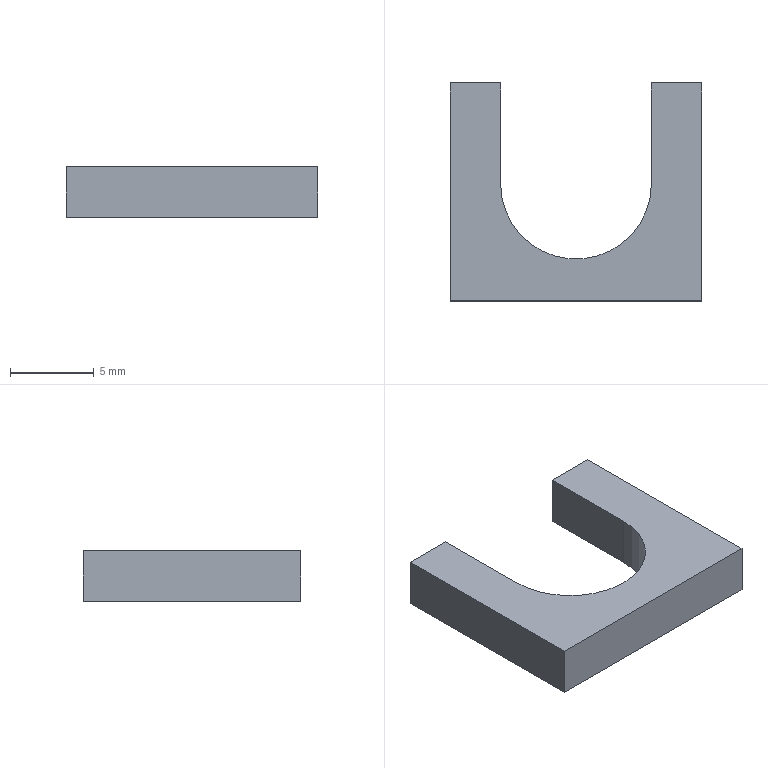Part | NX | features BREP 1 | 1 solid | 10 faces | box 15 x 13 x 3 mm | volume 327.574 mm3 | plane 9 | cylinder 1 | commonest cylinder face diameters 9 x1
STEP:
#1=CARTESIAN_POINT('',(-7.5,13.,0.));
#2=VERTEX_POINT('',#1);
#3=CARTESIAN_POINT('',(-7.5,0.,0.));
#4=VERTEX_POINT('',#3);
#5=CARTESIAN_POINT('',(-7.5,13.,0.));
#6=DIRECTION('',(0.,-1.,0.));
#7=VECTOR('',#6,1000.);
#8=LINE('',#5,#7);
#9=EDGE_CURVE('',#2,#4,#8,.T.);
#10=ORIENTED_EDGE('',*,*,#9,.T.);
#11=CARTESIAN_POINT('',(-7.5,0.,3.));
#12=VERTEX_POINT('',#11);
#13=CARTESIAN_POINT('',(-7.5,0.,3.));
#14=DIRECTION('',(0.,0.,-1.));
#15=VECTOR('',#14,1000.);
#16=LINE('',#13,#15);
#17=EDGE_CURVE('',#12,#4,#16,.T.);
#18=ORIENTED_EDGE('',*,*,#17,.F.);
#19=CARTESIAN_POINT('',(-7.5,13.,3.));
#20=VERTEX_POINT('',#19);
#21=CARTESIAN_POINT('',(-7.5,13.,3.));
#22=DIRECTION('',(0.,-1.,0.));
#23=VECTOR('',#22,1000.);
#24=LINE('',#21,#23);
#25=EDGE_CURVE('',#20,#12,#24,.T.);
#26=ORIENTED_EDGE('',*,*,#25,.F.);
#27=CARTESIAN_POINT('',(-7.5,13.,3.));
#28=DIRECTION('',(0.,0.,-1.));
#29=VECTOR('',#28,1000.);
#30=LINE('',#27,#29);
#31=EDGE_CURVE('',#20,#2,#30,.T.);
#32=ORIENTED_EDGE('',*,*,#31,.T.);
#33=EDGE_LOOP('',(#10,#18,#26,#32));
#34=FACE_BOUND('',#33,.T.);
#35=CARTESIAN_POINT('',(-7.5,13.,3.));
#36=DIRECTION('',(1.,0.,0.));
#37=DIRECTION('',(0.,-1.,0.));
#38=AXIS2_PLACEMENT_3D('',#35,#36,#37);
#39=PLANE('',#38);
#40=ADVANCED_FACE('',(#34),#39,.F.);
#41=CARTESIAN_POINT('',(7.5,0.,0.));
#42=VERTEX_POINT('',#41);
#43=CARTESIAN_POINT('',(-7.5,0.,0.));
#44=DIRECTION('',(1.,0.,0.));
#45=VECTOR('',#44,1000.);
#46=LINE('',#43,#45);
#47=EDGE_CURVE('',#4,#42,#46,.T.);
#48=ORIENTED_EDGE('',*,*,#47,.T.);
#49=CARTESIAN_POINT('',(7.5,0.,3.));
#50=VERTEX_POINT('',#49);
#51=CARTESIAN_POINT('',(7.5,0.,3.));
#52=DIRECTION('',(0.,0.,-1.));
#53=VECTOR('',#52,1000.);
#54=LINE('',#51,#53);
#55=EDGE_CURVE('',#50,#42,#54,.T.);
#56=ORIENTED_EDGE('',*,*,#55,.F.);
#57=CARTESIAN_POINT('',(-7.5,0.,3.));
#58=DIRECTION('',(1.,0.,0.));
#59=VECTOR('',#58,1000.);
#60=LINE('',#57,#59);
#61=EDGE_CURVE('',#12,#50,#60,.T.);
#62=ORIENTED_EDGE('',*,*,#61,.F.);
#63=ORIENTED_EDGE('',*,*,#17,.T.);
#64=EDGE_LOOP('',(#48,#56,#62,#63));
#65=FACE_BOUND('',#64,.T.);
#66=CARTESIAN_POINT('',(-7.5,0.,3.));
#67=DIRECTION('',(0.,1.,0.));
#68=DIRECTION('',(0.,0.,-1.));
#69=AXIS2_PLACEMENT_3D('',#66,#67,#68);
#70=PLANE('',#69);
#71=ADVANCED_FACE('',(#65),#70,.F.);
#72=CARTESIAN_POINT('',(7.5,13.,0.));
#73=VERTEX_POINT('',#72);
#74=CARTESIAN_POINT('',(7.5,0.,0.));
#75=DIRECTION('',(0.,1.,0.));
#76=VECTOR('',#75,1000.);
#77=LINE('',#74,#76);
#78=EDGE_CURVE('',#42,#73,#77,.T.);
#79=ORIENTED_EDGE('',*,*,#78,.T.);
#80=CARTESIAN_POINT('',(7.5,13.,3.));
#81=VERTEX_POINT('',#80);
#82=CARTESIAN_POINT('',(7.5,13.,3.));
#83=DIRECTION('',(0.,0.,-1.));
#84=VECTOR('',#83,1000.);
#85=LINE('',#82,#84);
#86=EDGE_CURVE('',#81,#73,#85,.T.);
#87=ORIENTED_EDGE('',*,*,#86,.F.);
#88=CARTESIAN_POINT('',(7.5,0.,3.));
#89=DIRECTION('',(0.,1.,0.));
#90=VECTOR('',#89,1000.);
#91=LINE('',#88,#90);
#92=EDGE_CURVE('',#50,#81,#91,.T.);
#93=ORIENTED_EDGE('',*,*,#92,.F.);
#94=ORIENTED_EDGE('',*,*,#55,.T.);
#95=EDGE_LOOP('',(#79,#87,#93,#94));
#96=FACE_BOUND('',#95,.T.);
#97=CARTESIAN_POINT('',(7.5,0.,3.));
#98=DIRECTION('',(-1.,0.,0.));
#99=DIRECTION('',(0.,1.,0.));
#100=AXIS2_PLACEMENT_3D('',#97,#98,#99);
#101=PLANE('',#100);
#102=ADVANCED_FACE('',(#96),#101,.F.);
#103=CARTESIAN_POINT('',(4.5,13.,0.));
#104=VERTEX_POINT('',#103);
#105=CARTESIAN_POINT('',(7.5,13.,0.));
#106=DIRECTION('',(-1.,0.,0.));
#107=VECTOR('',#106,1000.);
#108=LINE('',#105,#107);
#109=EDGE_CURVE('',#73,#104,#108,.T.);
#110=ORIENTED_EDGE('',*,*,#109,.T.);
#111=CARTESIAN_POINT('',(4.5,13.,3.));
#112=VERTEX_POINT('',#111);
#113=CARTESIAN_POINT('',(4.5,13.,3.));
#114=DIRECTION('',(0.,0.,-1.));
#115=VECTOR('',#114,1000.);
#116=LINE('',#113,#115);
#117=EDGE_CURVE('',#112,#104,#116,.T.);
#118=ORIENTED_EDGE('',*,*,#117,.F.);
#119=CARTESIAN_POINT('',(7.5,13.,3.));
#120=DIRECTION('',(-1.,0.,0.));
#121=VECTOR('',#120,1000.);
#122=LINE('',#119,#121);
#123=EDGE_CURVE('',#81,#112,#122,.T.);
#124=ORIENTED_EDGE('',*,*,#123,.F.);
#125=ORIENTED_EDGE('',*,*,#86,.T.);
#126=EDGE_LOOP('',(#110,#118,#124,#125));
#127=FACE_BOUND('',#126,.T.);
#128=CARTESIAN_POINT('',(7.5,13.,3.));
#129=DIRECTION('',(0.,-1.,0.));
#130=DIRECTION('',(0.,0.,1.));
#131=AXIS2_PLACEMENT_3D('',#128,#129,#130);
#132=PLANE('',#131);
#133=ADVANCED_FACE('',(#127),#132,.F.);
#134=CARTESIAN_POINT('',(4.5,7.,0.));
#135=VERTEX_POINT('',#134);
#136=CARTESIAN_POINT('',(4.5,13.,0.));
#137=DIRECTION('',(0.,-1.,0.));
#138=VECTOR('',#137,1000.);
#139=LINE('',#136,#138);
#140=EDGE_CURVE('',#104,#135,#139,.T.);
#141=ORIENTED_EDGE('',*,*,#140,.T.);
#142=CARTESIAN_POINT('',(4.5,7.,3.));
#143=VERTEX_POINT('',#142);
#144=CARTESIAN_POINT('',(4.5,7.,3.));
#145=DIRECTION('',(0.,0.,-1.));
#146=VECTOR('',#145,1000.);
#147=LINE('',#144,#146);
#148=EDGE_CURVE('',#143,#135,#147,.T.);
#149=ORIENTED_EDGE('',*,*,#148,.F.);
#150=CARTESIAN_POINT('',(4.5,13.,3.));
#151=DIRECTION('',(0.,-1.,0.));
#152=VECTOR('',#151,1000.);
#153=LINE('',#150,#152);
#154=EDGE_CURVE('',#112,#143,#153,.T.);
#155=ORIENTED_EDGE('',*,*,#154,.F.);
#156=ORIENTED_EDGE('',*,*,#117,.T.);
#157=EDGE_LOOP('',(#141,#149,#155,#156));
#158=FACE_BOUND('',#157,.T.);
#159=CARTESIAN_POINT('',(4.5,13.,3.));
#160=DIRECTION('',(1.,0.,0.));
#161=DIRECTION('',(0.,-1.,0.));
#162=AXIS2_PLACEMENT_3D('',#159,#160,#161);
#163=PLANE('',#162);
#164=ADVANCED_FACE('',(#158),#163,.F.);
#165=CARTESIAN_POINT('',(-4.5,7.,0.));
#166=VERTEX_POINT('',#165);
#167=CARTESIAN_POINT('',(0.,7.,0.));
#168=DIRECTION('',(0.,0.,-1.));
#169=DIRECTION('',(-1.,0.,0.));
#170=AXIS2_PLACEMENT_3D('',#167,#168,#169);
#171=CIRCLE('',#170,4.5);
#172=EDGE_CURVE('',#135,#166,#171,.T.);
#173=ORIENTED_EDGE('',*,*,#172,.T.);
#174=CARTESIAN_POINT('',(-4.5,7.,3.));
#175=VERTEX_POINT('',#174);
#176=CARTESIAN_POINT('',(-4.5,7.,3.));
#177=DIRECTION('',(0.,0.,-1.));
#178=VECTOR('',#177,1000.);
#179=LINE('',#176,#178);
#180=EDGE_CURVE('',#175,#166,#179,.T.);
#181=ORIENTED_EDGE('',*,*,#180,.F.);
#182=CARTESIAN_POINT('',(0.,7.,3.));
#183=DIRECTION('',(0.,0.,-1.));
#184=DIRECTION('',(-1.,0.,0.));
#185=AXIS2_PLACEMENT_3D('',#182,#183,#184);
#186=CIRCLE('',#185,4.5);
#187=EDGE_CURVE('',#143,#175,#186,.T.);
#188=ORIENTED_EDGE('',*,*,#187,.F.);
#189=ORIENTED_EDGE('',*,*,#148,.T.);
#190=EDGE_LOOP('',(#173,#181,#188,#189));
#191=FACE_BOUND('',#190,.T.);
#192=CARTESIAN_POINT('',(0.,7.,3.));
#193=DIRECTION('',(0.,0.,-1.));
#194=DIRECTION('',(1.,0.,0.));
#195=AXIS2_PLACEMENT_3D('',#192,#193,#194);
#196=CYLINDRICAL_SURFACE('',#195,4.5);
#197=ADVANCED_FACE('',(#191),#196,.F.);
#198=CARTESIAN_POINT('',(-4.5,13.,0.));
#199=VERTEX_POINT('',#198);
#200=CARTESIAN_POINT('',(-4.5,7.,0.));
#201=DIRECTION('',(0.,1.,0.));
#202=VECTOR('',#201,1000.);
#203=LINE('',#200,#202);
#204=EDGE_CURVE('',#166,#199,#203,.T.);
#205=ORIENTED_EDGE('',*,*,#204,.T.);
#206=CARTESIAN_POINT('',(-4.5,13.,3.));
#207=VERTEX_POINT('',#206);
#208=CARTESIAN_POINT('',(-4.5,13.,3.));
#209=DIRECTION('',(0.,0.,-1.));
#210=VECTOR('',#209,1000.);
#211=LINE('',#208,#210);
#212=EDGE_CURVE('',#207,#199,#211,.T.);
#213=ORIENTED_EDGE('',*,*,#212,.F.);
#214=CARTESIAN_POINT('',(-4.5,7.,3.));
#215=DIRECTION('',(0.,1.,0.));
#216=VECTOR('',#215,1000.);
#217=LINE('',#214,#216);
#218=EDGE_CURVE('',#175,#207,#217,.T.);
#219=ORIENTED_EDGE('',*,*,#218,.F.);
#220=ORIENTED_EDGE('',*,*,#180,.T.);
#221=EDGE_LOOP('',(#205,#213,#219,#220));
#222=FACE_BOUND('',#221,.T.);
#223=CARTESIAN_POINT('',(-4.5,7.,3.));
#224=DIRECTION('',(-1.,0.,0.));
#225=DIRECTION('',(0.,0.,-1.));
#226=AXIS2_PLACEMENT_3D('',#223,#224,#225);
#227=PLANE('',#226);
#228=ADVANCED_FACE('',(#222),#227,.F.);
#229=CARTESIAN_POINT('',(-4.5,13.,0.));
#230=DIRECTION('',(-1.,0.,0.));
#231=VECTOR('',#230,1000.);
#232=LINE('',#229,#231);
#233=EDGE_CURVE('',#199,#2,#232,.T.);
#234=ORIENTED_EDGE('',*,*,#233,.T.);
#235=ORIENTED_EDGE('',*,*,#31,.F.);
#236=CARTESIAN_POINT('',(-4.5,13.,3.));
#237=DIRECTION('',(-1.,0.,0.));
#238=VECTOR('',#237,1000.);
#239=LINE('',#236,#238);
#240=EDGE_CURVE('',#207,#20,#239,.T.);
#241=ORIENTED_EDGE('',*,*,#240,.F.);
#242=ORIENTED_EDGE('',*,*,#212,.T.);
#243=EDGE_LOOP('',(#234,#235,#241,#242));
#244=FACE_BOUND('',#243,.T.);
#245=CARTESIAN_POINT('',(-4.5,13.,3.));
#246=DIRECTION('',(0.,-1.,0.));
#247=DIRECTION('',(0.,0.,1.));
#248=AXIS2_PLACEMENT_3D('',#245,#246,#247);
#249=PLANE('',#248);
#250=ADVANCED_FACE('',(#244),#249,.F.);
#251=ORIENTED_EDGE('',*,*,#25,.T.);
#252=ORIENTED_EDGE('',*,*,#61,.T.);
#253=ORIENTED_EDGE('',*,*,#92,.T.);
#254=ORIENTED_EDGE('',*,*,#123,.T.);
#255=ORIENTED_EDGE('',*,*,#154,.T.);
#256=ORIENTED_EDGE('',*,*,#187,.T.);
#257=ORIENTED_EDGE('',*,*,#218,.T.);
#258=ORIENTED_EDGE('',*,*,#240,.T.);
#259=EDGE_LOOP('',(#251,#252,#253,#254,#255,#256,#257,#258));
#260=FACE_BOUND('',#259,.T.);
#261=CARTESIAN_POINT('',(0.,7.,3.));
#262=DIRECTION('',(0.,0.,-1.));
#263=DIRECTION('',(1.,0.,0.));
#264=AXIS2_PLACEMENT_3D('',#261,#262,#263);
#265=PLANE('',#264);
#266=ADVANCED_FACE('',(#260),#265,.F.);
#267=ORIENTED_EDGE('',*,*,#9,.F.);
#268=ORIENTED_EDGE('',*,*,#233,.F.);
#269=ORIENTED_EDGE('',*,*,#204,.F.);
#270=ORIENTED_EDGE('',*,*,#172,.F.);
#271=ORIENTED_EDGE('',*,*,#140,.F.);
#272=ORIENTED_EDGE('',*,*,#109,.F.);
#273=ORIENTED_EDGE('',*,*,#78,.F.);
#274=ORIENTED_EDGE('',*,*,#47,.F.);
#275=EDGE_LOOP('',(#267,#268,#269,#270,#271,#272,#273,#274));
#276=FACE_BOUND('',#275,.T.);
#277=CARTESIAN_POINT('',(0.,7.,0.));
#278=DIRECTION('',(0.,0.,-1.));
#279=DIRECTION('',(1.,0.,0.));
#280=AXIS2_PLACEMENT_3D('',#277,#278,#279);
#281=PLANE('',#280);
#282=ADVANCED_FACE('',(#276),#281,.T.);
#283=CLOSED_SHELL('',(#40,#71,#102,#133,#164,#197,#228,#250,#266,#282));
#284=MANIFOLD_SOLID_BREP('',#283);
#285=(LENGTH_UNIT()NAMED_UNIT(*)SI_UNIT(.MILLI.,.METRE.));
#286=UNCERTAINTY_MEASURE_WITH_UNIT(LENGTH_MEASURE(0.00001),#285,'','');
#287=(NAMED_UNIT(*)PLANE_ANGLE_UNIT()SI_UNIT($,.RADIAN.));
#288=(NAMED_UNIT(*)SI_UNIT($,.STERADIAN.)SOLID_ANGLE_UNIT());
#289=(GEOMETRIC_REPRESENTATION_CONTEXT(3)GLOBAL_UNCERTAINTY_ASSIGNED_CONTEXT((#286))GLOBAL_UNIT_ASSIGNED_CONTEXT((#285,#287,#288))REPRESENTATION_CONTEXT('',''));
#290=ADVANCED_BREP_SHAPE_REPRESENTATION('',(#284),#289);